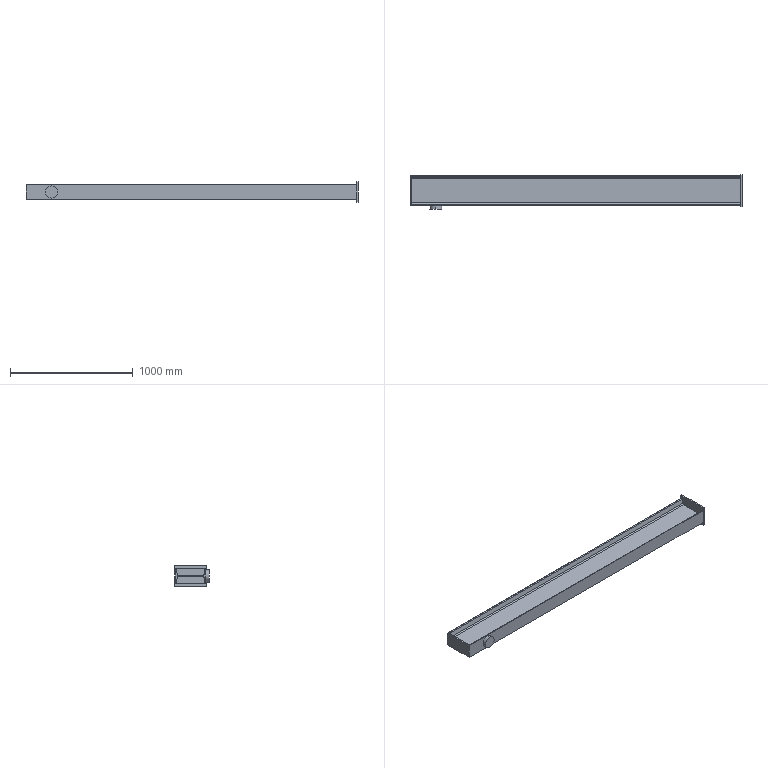Part | SolidWorks | features ICE 3, Fillet 2, Extrusion 1 | 1 solid | 30 faces | box 2710 x 284 x 170 mm | volume 14871084 mm3 | plane 20 | cylinder 10 | commonest cylinder face diameters 10 x4 20 x4 100 x2
STEP:
#1=CARTESIAN_POINT('',(205.,-28.,-50.));
#2=VERTEX_POINT('',#1);
#3=CARTESIAN_POINT('',(205.,-28.,50.));
#4=VERTEX_POINT('',#3);
#5=CARTESIAN_POINT('',(205.,-28.,0.));
#6=DIRECTION('',(0.,-1.,0.));
#7=DIRECTION('',(0.,0.,-1.));
#8=AXIS2_PLACEMENT_3D('',#5,#6,#7);
#9=CIRCLE('',#8,50.);
#10=EDGE_CURVE('',#2,#4,#9,.T.);
#11=ORIENTED_EDGE('',*,*,#10,.F.);
#12=CARTESIAN_POINT('',(205.,0.,-50.));
#13=VERTEX_POINT('',#12);
#14=CARTESIAN_POINT('',(205.,-28.,-50.));
#15=DIRECTION('',(0.,1.,0.));
#16=VECTOR('',#15,1000.);
#17=LINE('',#14,#16);
#18=EDGE_CURVE('',#2,#13,#17,.T.);
#19=ORIENTED_EDGE('',*,*,#18,.T.);
#20=CARTESIAN_POINT('',(205.,0.,50.));
#21=VERTEX_POINT('',#20);
#22=CARTESIAN_POINT('',(205.,0.,0.));
#23=DIRECTION('',(0.,-1.,0.));
#24=DIRECTION('',(0.,0.,1.));
#25=AXIS2_PLACEMENT_3D('',#22,#23,#24);
#26=CIRCLE('',#25,50.);
#27=EDGE_CURVE('',#13,#21,#26,.T.);
#28=ORIENTED_EDGE('',*,*,#27,.T.);
#29=CARTESIAN_POINT('',(205.,-28.,50.));
#30=DIRECTION('',(0.,1.,0.));
#31=VECTOR('',#30,1000.);
#32=LINE('',#29,#31);
#33=EDGE_CURVE('',#4,#21,#32,.T.);
#34=ORIENTED_EDGE('',*,*,#33,.F.);
#35=EDGE_LOOP('',(#11,#19,#28,#34));
#36=FACE_OUTER_BOUND('',#35,.T.);
#37=CARTESIAN_POINT('',(205.,-28.,0.));
#38=DIRECTION('',(0.,1.,0.));
#39=DIRECTION('',(0.,0.,1.));
#40=AXIS2_PLACEMENT_3D('',#37,#38,#39);
#41=CYLINDRICAL_SURFACE('',#40,50.);
#42=ADVANCED_FACE('',(#36),#41,.T.);
#43=CARTESIAN_POINT('',(2695.,8.363,-54.822));
#44=VERTEX_POINT('',#43);
#45=CARTESIAN_POINT('',(2695.,15.274,-13.356));
#46=VERTEX_POINT('',#45);
#47=CARTESIAN_POINT('',(2695.,16.667,-5.));
#48=DIRECTION('',(0.,0.1644,0.9864));
#49=VECTOR('',#48,1000.);
#50=LINE('',#47,#49);
#51=EDGE_CURVE('',#44,#46,#50,.T.);
#52=ORIENTED_EDGE('',*,*,#51,.F.);
#53=CARTESIAN_POINT('',(5.,8.363,-54.822));
#54=VERTEX_POINT('',#53);
#55=CARTESIAN_POINT('',(2700.,8.363,-54.822));
#56=DIRECTION('',(-1.,0.,0.));
#57=VECTOR('',#56,1000.);
#58=LINE('',#55,#57);
#59=EDGE_CURVE('',#44,#54,#58,.T.);
#60=ORIENTED_EDGE('',*,*,#59,.T.);
#61=CARTESIAN_POINT('',(5.,15.274,-13.356));
#62=VERTEX_POINT('',#61);
#63=CARTESIAN_POINT('',(5.,16.667,-5.));
#64=DIRECTION('',(0.,-0.1644,-0.9864));
#65=VECTOR('',#64,1000.);
#66=LINE('',#63,#65);
#67=EDGE_CURVE('',#62,#54,#66,.T.);
#68=ORIENTED_EDGE('',*,*,#67,.F.);
#69=CARTESIAN_POINT('',(2700.,15.274,-13.356));
#70=DIRECTION('',(1.,0.,0.));
#71=VECTOR('',#70,1000.);
#72=LINE('',#69,#71);
#73=EDGE_CURVE('',#62,#46,#72,.T.);
#74=ORIENTED_EDGE('',*,*,#73,.T.);
#75=EDGE_LOOP('',(#52,#60,#68,#74));
#76=FACE_OUTER_BOUND('',#75,.T.);
#77=CARTESIAN_POINT('',(2700.,16.667,-5.));
#78=DIRECTION('',(0.,-0.9864,0.1644));
#79=DIRECTION('',(0.,-0.1644,-0.9864));
#80=AXIS2_PLACEMENT_3D('',#77,#78,#79);
#81=PLANE('',#80);
#82=ADVANCED_FACE('',(#76),#81,.F.);
#83=CARTESIAN_POINT('',(2695.,25.138,-5.));
#84=VERTEX_POINT('',#83);
#85=CARTESIAN_POINT('',(2695.,224.862,-5.));
#86=VERTEX_POINT('',#85);
#87=CARTESIAN_POINT('',(2695.,233.333,-5.));
#88=DIRECTION('',(0.,1.,0.));
#89=VECTOR('',#88,1000.);
#90=LINE('',#87,#89);
#91=EDGE_CURVE('',#84,#86,#90,.T.);
#92=ORIENTED_EDGE('',*,*,#91,.F.);
#93=CARTESIAN_POINT('',(5.,25.138,-5.));
#94=VERTEX_POINT('',#93);
#95=CARTESIAN_POINT('',(0.,25.138,-5.));
#96=DIRECTION('',(-1.,0.,0.));
#97=VECTOR('',#96,1000.);
#98=LINE('',#95,#97);
#99=EDGE_CURVE('',#84,#94,#98,.T.);
#100=ORIENTED_EDGE('',*,*,#99,.T.);
#101=CARTESIAN_POINT('',(5.,224.862,-5.));
#102=VERTEX_POINT('',#101);
#103=CARTESIAN_POINT('',(5.,233.333,-5.));
#104=DIRECTION('',(0.,-1.,0.));
#105=VECTOR('',#104,1000.);
#106=LINE('',#103,#105);
#107=EDGE_CURVE('',#102,#94,#106,.T.);
#108=ORIENTED_EDGE('',*,*,#107,.F.);
#109=CARTESIAN_POINT('',(2700.,224.862,-5.));
#110=DIRECTION('',(1.,0.,0.));
#111=VECTOR('',#110,1000.);
#112=LINE('',#109,#111);
#113=EDGE_CURVE('',#102,#86,#112,.T.);
#114=ORIENTED_EDGE('',*,*,#113,.T.);
#115=EDGE_LOOP('',(#92,#100,#108,#114));
#116=FACE_OUTER_BOUND('',#115,.T.);
#117=CARTESIAN_POINT('',(2700.,233.333,-5.));
#118=DIRECTION('',(0.,0.,1.));
#119=DIRECTION('',(0.,-1.,0.));
#120=AXIS2_PLACEMENT_3D('',#117,#118,#119);
#121=PLANE('',#120);
#122=ADVANCED_FACE('',(#116),#121,.F.);
#123=CARTESIAN_POINT('',(2695.,234.726,-13.356));
#124=VERTEX_POINT('',#123);
#125=CARTESIAN_POINT('',(2695.,241.637,-54.822));
#126=VERTEX_POINT('',#125);
#127=CARTESIAN_POINT('',(2695.,242.333,-59.));
#128=DIRECTION('',(0.,0.1644,-0.9864));
#129=VECTOR('',#128,1000.);
#130=LINE('',#127,#129);
#131=EDGE_CURVE('',#124,#126,#130,.T.);
#132=ORIENTED_EDGE('',*,*,#131,.F.);
#133=CARTESIAN_POINT('',(5.,234.726,-13.356));
#134=VERTEX_POINT('',#133);
#135=CARTESIAN_POINT('',(0.,234.726,-13.356));
#136=DIRECTION('',(-1.,0.,0.));
#137=VECTOR('',#136,1000.);
#138=LINE('',#135,#137);
#139=EDGE_CURVE('',#124,#134,#138,.T.);
#140=ORIENTED_EDGE('',*,*,#139,.T.);
#141=CARTESIAN_POINT('',(5.,241.637,-54.822));
#142=VERTEX_POINT('',#141);
#143=CARTESIAN_POINT('',(5.,242.333,-59.));
#144=DIRECTION('',(0.,-0.1644,0.9864));
#145=VECTOR('',#144,1000.);
#146=LINE('',#143,#145);
#147=EDGE_CURVE('',#142,#134,#146,.T.);
#148=ORIENTED_EDGE('',*,*,#147,.F.);
#149=CARTESIAN_POINT('',(2700.,241.637,-54.822));
#150=DIRECTION('',(1.,0.,0.));
#151=VECTOR('',#150,1000.);
#152=LINE('',#149,#151);
#153=EDGE_CURVE('',#142,#126,#152,.T.);
#154=ORIENTED_EDGE('',*,*,#153,.T.);
#155=EDGE_LOOP('',(#132,#140,#148,#154));
#156=FACE_OUTER_BOUND('',#155,.T.);
#157=CARTESIAN_POINT('',(2700.,242.333,-59.));
#158=DIRECTION('',(0.,0.9864,0.1644));
#159=DIRECTION('',(0.,-0.1644,0.9864));
#160=AXIS2_PLACEMENT_3D('',#157,#158,#159);
#161=PLANE('',#160);
#162=ADVANCED_FACE('',(#156),#161,.F.);
#163=CARTESIAN_POINT('',(2695.,241.637,54.822));
#164=VERTEX_POINT('',#163);
#165=CARTESIAN_POINT('',(2695.,234.726,13.356));
#166=VERTEX_POINT('',#165);
#167=CARTESIAN_POINT('',(2695.,242.333,59.));
#168=DIRECTION('',(0.,-0.1644,-0.9864));
#169=VECTOR('',#168,1000.);
#170=LINE('',#167,#169);
#171=EDGE_CURVE('',#164,#166,#170,.T.);
#172=ORIENTED_EDGE('',*,*,#171,.F.);
#173=CARTESIAN_POINT('',(5.,241.637,54.822));
#174=VERTEX_POINT('',#173);
#175=CARTESIAN_POINT('',(2700.,241.637,54.822));
#176=DIRECTION('',(-1.,0.,0.));
#177=VECTOR('',#176,1000.);
#178=LINE('',#175,#177);
#179=EDGE_CURVE('',#164,#174,#178,.T.);
#180=ORIENTED_EDGE('',*,*,#179,.T.);
#181=CARTESIAN_POINT('',(5.,234.726,13.356));
#182=VERTEX_POINT('',#181);
#183=CARTESIAN_POINT('',(5.,242.333,59.));
#184=DIRECTION('',(0.,0.1644,0.9864));
#185=VECTOR('',#184,1000.);
#186=LINE('',#183,#185);
#187=EDGE_CURVE('',#182,#174,#186,.T.);
#188=ORIENTED_EDGE('',*,*,#187,.F.);
#189=CARTESIAN_POINT('',(2700.,234.726,13.356));
#190=DIRECTION('',(1.,0.,0.));
#191=VECTOR('',#190,1000.);
#192=LINE('',#189,#191);
#193=EDGE_CURVE('',#182,#166,#192,.T.);
#194=ORIENTED_EDGE('',*,*,#193,.T.);
#195=EDGE_LOOP('',(#172,#180,#188,#194));
#196=FACE_OUTER_BOUND('',#195,.T.);
#197=CARTESIAN_POINT('',(2700.,242.333,59.));
#198=DIRECTION('',(0.,0.9864,-0.1644));
#199=DIRECTION('',(0.,0.1644,0.9864));
#200=AXIS2_PLACEMENT_3D('',#197,#198,#199);
#201=PLANE('',#200);
#202=ADVANCED_FACE('',(#196),#201,.F.);
#203=CARTESIAN_POINT('',(2695.,224.862,5.));
#204=VERTEX_POINT('',#203);
#205=CARTESIAN_POINT('',(2695.,25.138,5.));
#206=VERTEX_POINT('',#205);
#207=CARTESIAN_POINT('',(2695.,233.333,5.));
#208=DIRECTION('',(0.,-1.,0.));
#209=VECTOR('',#208,1000.);
#210=LINE('',#207,#209);
#211=EDGE_CURVE('',#204,#206,#210,.T.);
#212=ORIENTED_EDGE('',*,*,#211,.F.);
#213=CARTESIAN_POINT('',(5.,224.862,5.));
#214=VERTEX_POINT('',#213);
#215=CARTESIAN_POINT('',(0.,224.862,5.));
#216=DIRECTION('',(-1.,0.,0.));
#217=VECTOR('',#216,1000.);
#218=LINE('',#215,#217);
#219=EDGE_CURVE('',#204,#214,#218,.T.);
#220=ORIENTED_EDGE('',*,*,#219,.T.);
#221=CARTESIAN_POINT('',(5.,25.138,5.));
#222=VERTEX_POINT('',#221);
#223=CARTESIAN_POINT('',(5.,233.333,5.));
#224=DIRECTION('',(0.,1.,0.));
#225=VECTOR('',#224,1000.);
#226=LINE('',#223,#225);
#227=EDGE_CURVE('',#222,#214,#226,.T.);
#228=ORIENTED_EDGE('',*,*,#227,.F.);
#229=CARTESIAN_POINT('',(2700.,25.138,5.));
#230=DIRECTION('',(1.,0.,0.));
#231=VECTOR('',#230,1000.);
#232=LINE('',#229,#231);
#233=EDGE_CURVE('',#222,#206,#232,.T.);
#234=ORIENTED_EDGE('',*,*,#233,.T.);
#235=EDGE_LOOP('',(#212,#220,#228,#234));
#236=FACE_OUTER_BOUND('',#235,.T.);
#237=CARTESIAN_POINT('',(2700.,233.333,5.));
#238=DIRECTION('',(0.,0.,-1.));
#239=DIRECTION('',(0.,1.,0.));
#240=AXIS2_PLACEMENT_3D('',#237,#238,#239);
#241=PLANE('',#240);
#242=ADVANCED_FACE('',(#236),#241,.F.);
#243=CARTESIAN_POINT('',(2695.,15.274,13.356));
#244=VERTEX_POINT('',#243);
#245=CARTESIAN_POINT('',(2695.,8.363,54.822));
#246=VERTEX_POINT('',#245);
#247=CARTESIAN_POINT('',(2695.,16.667,5.));
#248=DIRECTION('',(0.,-0.1644,0.9864));
#249=VECTOR('',#248,1000.);
#250=LINE('',#247,#249);
#251=EDGE_CURVE('',#244,#246,#250,.T.);
#252=ORIENTED_EDGE('',*,*,#251,.F.);
#253=CARTESIAN_POINT('',(5.,15.274,13.356));
#254=VERTEX_POINT('',#253);
#255=CARTESIAN_POINT('',(0.,15.274,13.356));
#256=DIRECTION('',(-1.,0.,0.));
#257=VECTOR('',#256,1000.);
#258=LINE('',#255,#257);
#259=EDGE_CURVE('',#244,#254,#258,.T.);
#260=ORIENTED_EDGE('',*,*,#259,.T.);
#261=CARTESIAN_POINT('',(5.,8.363,54.822));
#262=VERTEX_POINT('',#261);
#263=CARTESIAN_POINT('',(5.,16.667,5.));
#264=DIRECTION('',(0.,0.1644,-0.9864));
#265=VECTOR('',#264,1000.);
#266=LINE('',#263,#265);
#267=EDGE_CURVE('',#262,#254,#266,.T.);
#268=ORIENTED_EDGE('',*,*,#267,.F.);
#269=CARTESIAN_POINT('',(2700.,8.363,54.822));
#270=DIRECTION('',(1.,0.,0.));
#271=VECTOR('',#270,1000.);
#272=LINE('',#269,#271);
#273=EDGE_CURVE('',#262,#246,#272,.T.);
#274=ORIENTED_EDGE('',*,*,#273,.T.);
#275=EDGE_LOOP('',(#252,#260,#268,#274));
#276=FACE_OUTER_BOUND('',#275,.T.);
#277=CARTESIAN_POINT('',(2700.,16.667,5.));
#278=DIRECTION('',(0.,-0.9864,-0.1644));
#279=DIRECTION('',(0.,0.1644,-0.9864));
#280=AXIS2_PLACEMENT_3D('',#277,#278,#279);
#281=PLANE('',#280);
#282=ADVANCED_FACE('',(#276),#281,.F.);
#283=CARTESIAN_POINT('',(2695.,224.862,-15.));
#284=DIRECTION('',(-1.,0.,0.));
#285=DIRECTION('',(0.,0.,-1.));
#286=AXIS2_PLACEMENT_3D('',#283,#284,#285);
#287=CIRCLE('',#286,10.);
#288=EDGE_CURVE('',#86,#124,#287,.T.);
#289=ORIENTED_EDGE('',*,*,#288,.F.);
#290=ORIENTED_EDGE('',*,*,#113,.F.);
#291=CARTESIAN_POINT('',(5.,224.862,-15.));
#292=DIRECTION('',(1.,0.,0.));
#293=DIRECTION('',(0.,0.,1.));
#294=AXIS2_PLACEMENT_3D('',#291,#292,#293);
#295=CIRCLE('',#294,10.);
#296=EDGE_CURVE('',#134,#102,#295,.T.);
#297=ORIENTED_EDGE('',*,*,#296,.F.);
#298=ORIENTED_EDGE('',*,*,#139,.F.);
#299=EDGE_LOOP('',(#289,#290,#297,#298));
#300=FACE_OUTER_BOUND('',#299,.T.);
#301=CARTESIAN_POINT('',(2700.,224.862,-15.));
#302=DIRECTION('',(1.,0.,0.));
#303=DIRECTION('',(0.,0.,-1.));
#304=AXIS2_PLACEMENT_3D('',#301,#302,#303);
#305=CYLINDRICAL_SURFACE('',#304,10.);
#306=ADVANCED_FACE('',(#300),#305,.F.);
#307=CARTESIAN_POINT('',(2695.,25.138,-15.));
#308=DIRECTION('',(-1.,0.,0.));
#309=DIRECTION('',(0.,0.,-1.));
#310=AXIS2_PLACEMENT_3D('',#307,#308,#309);
#311=CIRCLE('',#310,10.);
#312=EDGE_CURVE('',#46,#84,#311,.T.);
#313=ORIENTED_EDGE('',*,*,#312,.F.);
#314=ORIENTED_EDGE('',*,*,#73,.F.);
#315=CARTESIAN_POINT('',(5.,25.138,-15.));
#316=DIRECTION('',(1.,0.,0.));
#317=DIRECTION('',(0.,0.,1.));
#318=AXIS2_PLACEMENT_3D('',#315,#316,#317);
#319=CIRCLE('',#318,10.);
#320=EDGE_CURVE('',#94,#62,#319,.T.);
#321=ORIENTED_EDGE('',*,*,#320,.F.);
#322=ORIENTED_EDGE('',*,*,#99,.F.);
#323=EDGE_LOOP('',(#313,#314,#321,#322));
#324=FACE_OUTER_BOUND('',#323,.T.);
#325=CARTESIAN_POINT('',(2700.,25.138,-15.));
#326=DIRECTION('',(1.,0.,0.));
#327=DIRECTION('',(0.,0.,-1.));
#328=AXIS2_PLACEMENT_3D('',#325,#326,#327);
#329=CYLINDRICAL_SURFACE('',#328,10.);
#330=ADVANCED_FACE('',(#324),#329,.F.);
#331=CARTESIAN_POINT('',(2695.,25.138,15.));
#332=DIRECTION('',(-1.,0.,0.));
#333=DIRECTION('',(0.,0.,-1.));
#334=AXIS2_PLACEMENT_3D('',#331,#332,#333);
#335=CIRCLE('',#334,10.);
#336=EDGE_CURVE('',#206,#244,#335,.T.);
#337=ORIENTED_EDGE('',*,*,#336,.F.);
#338=ORIENTED_EDGE('',*,*,#233,.F.);
#339=CARTESIAN_POINT('',(5.,25.138,15.));
#340=DIRECTION('',(1.,0.,0.));
#341=DIRECTION('',(0.,0.,1.));
#342=AXIS2_PLACEMENT_3D('',#339,#340,#341);
#343=CIRCLE('',#342,10.);
#344=EDGE_CURVE('',#254,#222,#343,.T.);
#345=ORIENTED_EDGE('',*,*,#344,.F.);
#346=ORIENTED_EDGE('',*,*,#259,.F.);
#347=EDGE_LOOP('',(#337,#338,#345,#346));
#348=FACE_OUTER_BOUND('',#347,.T.);
#349=CARTESIAN_POINT('',(2700.,25.138,15.));
#350=DIRECTION('',(1.,0.,0.));
#351=DIRECTION('',(0.,0.,-1.));
#352=AXIS2_PLACEMENT_3D('',#349,#350,#351);
#353=CYLINDRICAL_SURFACE('',#352,10.);
#354=ADVANCED_FACE('',(#348),#353,.F.);
#355=CARTESIAN_POINT('',(2695.,224.862,15.));
#356=DIRECTION('',(-1.,0.,0.));
#357=DIRECTION('',(0.,0.,-1.));
#358=AXIS2_PLACEMENT_3D('',#355,#356,#357);
#359=CIRCLE('',#358,10.);
#360=EDGE_CURVE('',#166,#204,#359,.T.);
#361=ORIENTED_EDGE('',*,*,#360,.F.);
#362=ORIENTED_EDGE('',*,*,#193,.F.);
#363=CARTESIAN_POINT('',(5.,224.862,15.));
#364=DIRECTION('',(1.,0.,0.));
#365=DIRECTION('',(0.,0.,1.));
#366=AXIS2_PLACEMENT_3D('',#363,#364,#365);
#367=CIRCLE('',#366,10.);
#368=EDGE_CURVE('',#214,#182,#367,.T.);
#369=ORIENTED_EDGE('',*,*,#368,.F.);
#370=ORIENTED_EDGE('',*,*,#219,.F.);
#371=EDGE_LOOP('',(#361,#362,#369,#370));
#372=FACE_OUTER_BOUND('',#371,.T.);
#373=CARTESIAN_POINT('',(2700.,224.862,15.));
#374=DIRECTION('',(1.,0.,0.));
#375=DIRECTION('',(0.,0.,-1.));
#376=AXIS2_PLACEMENT_3D('',#373,#374,#375);
#377=CYLINDRICAL_SURFACE('',#376,10.);
#378=ADVANCED_FACE('',(#372),#377,.F.);
#379=ORIENTED_EDGE('',*,*,#179,.F.);
#380=CARTESIAN_POINT('',(2695.,246.569,59.));
#381=VERTEX_POINT('',#380);
#382=CARTESIAN_POINT('',(2695.,246.569,54.));
#383=DIRECTION('',(-1.,0.,0.));
#384=DIRECTION('',(0.,0.,-1.));
#385=AXIS2_PLACEMENT_3D('',#382,#383,#384);
#386=CIRCLE('',#385,5.);
#387=EDGE_CURVE('',#164,#381,#386,.T.);
#388=ORIENTED_EDGE('',*,*,#387,.T.);
#389=CARTESIAN_POINT('',(5.,246.569,59.));
#390=VERTEX_POINT('',#389);
#391=CARTESIAN_POINT('',(2700.,246.569,59.));
#392=DIRECTION('',(1.,0.,0.));
#393=VECTOR('',#392,1000.);
#394=LINE('',#391,#393);
#395=EDGE_CURVE('',#390,#381,#394,.T.);
#396=ORIENTED_EDGE('',*,*,#395,.F.);
#397=CARTESIAN_POINT('',(5.,246.569,54.));
#398=DIRECTION('',(1.,0.,0.));
#399=DIRECTION('',(0.,0.,1.));
#400=AXIS2_PLACEMENT_3D('',#397,#398,#399);
#401=CIRCLE('',#400,5.);
#402=EDGE_CURVE('',#390,#174,#401,.T.);
#403=ORIENTED_EDGE('',*,*,#402,.T.);
#404=EDGE_LOOP('',(#379,#388,#396,#403));
#405=FACE_OUTER_BOUND('',#404,.T.);
#406=CARTESIAN_POINT('',(2700.,246.569,54.));
#407=DIRECTION('',(-1.,0.,0.));
#408=DIRECTION('',(0.,0.,1.));
#409=AXIS2_PLACEMENT_3D('',#406,#407,#408);
#410=CYLINDRICAL_SURFACE('',#409,5.);
#411=ADVANCED_FACE('',(#405),#410,.T.);
#412=CARTESIAN_POINT('',(2695.,3.431,59.));
#413=VERTEX_POINT('',#412);
#414=CARTESIAN_POINT('',(5.,3.431,59.));
#415=VERTEX_POINT('',#414);
#416=CARTESIAN_POINT('',(2700.,3.431,59.));
#417=DIRECTION('',(-1.,0.,0.));
#418=VECTOR('',#417,1000.);
#419=LINE('',#416,#418);
#420=EDGE_CURVE('',#413,#415,#419,.T.);
#421=ORIENTED_EDGE('',*,*,#420,.F.);
#422=CARTESIAN_POINT('',(2695.,3.431,54.));
#423=DIRECTION('',(-1.,0.,0.));
#424=DIRECTION('',(0.,0.,-1.));
#425=AXIS2_PLACEMENT_3D('',#422,#423,#424);
#426=CIRCLE('',#425,5.);
#427=EDGE_CURVE('',#413,#246,#426,.T.);
#428=ORIENTED_EDGE('',*,*,#427,.T.);
#429=ORIENTED_EDGE('',*,*,#273,.F.);
#430=CARTESIAN_POINT('',(5.,3.431,54.));
#431=DIRECTION('',(1.,0.,0.));
#432=DIRECTION('',(0.,0.,1.));
#433=AXIS2_PLACEMENT_3D('',#430,#431,#432);
#434=CIRCLE('',#433,5.);
#435=EDGE_CURVE('',#262,#415,#434,.T.);
#436=ORIENTED_EDGE('',*,*,#435,.T.);
#437=EDGE_LOOP('',(#421,#428,#429,#436));
#438=FACE_OUTER_BOUND('',#437,.T.);
#439=CARTESIAN_POINT('',(2700.,3.431,54.));
#440=DIRECTION('',(-1.,0.,0.));
#441=DIRECTION('',(0.,0.,1.));
#442=AXIS2_PLACEMENT_3D('',#439,#440,#441);
#443=CYLINDRICAL_SURFACE('',#442,5.);
#444=ADVANCED_FACE('',(#438),#443,.T.);
#445=ORIENTED_EDGE('',*,*,#59,.F.);
#446=CARTESIAN_POINT('',(2695.,3.431,-59.));
#447=VERTEX_POINT('',#446);
#448=CARTESIAN_POINT('',(2695.,3.431,-54.));
#449=DIRECTION('',(-1.,0.,0.));
#450=DIRECTION('',(0.,0.,-1.));
#451=AXIS2_PLACEMENT_3D('',#448,#449,#450);
#452=CIRCLE('',#451,5.);
#453=EDGE_CURVE('',#44,#447,#452,.T.);
#454=ORIENTED_EDGE('',*,*,#453,.T.);
#455=CARTESIAN_POINT('',(5.,3.431,-59.));
#456=VERTEX_POINT('',#455);
#457=CARTESIAN_POINT('',(2700.,3.431,-59.));
#458=DIRECTION('',(1.,0.,0.));
#459=VECTOR('',#458,1000.);
#460=LINE('',#457,#459);
#461=EDGE_CURVE('',#456,#447,#460,.T.);
#462=ORIENTED_EDGE('',*,*,#461,.F.);
#463=CARTESIAN_POINT('',(5.,3.431,-54.));
#464=DIRECTION('',(1.,0.,0.));
#465=DIRECTION('',(0.,0.,1.));
#466=AXIS2_PLACEMENT_3D('',#463,#464,#465);
#467=CIRCLE('',#466,5.);
#468=EDGE_CURVE('',#456,#54,#467,.T.);
#469=ORIENTED_EDGE('',*,*,#468,.T.);
#470=EDGE_LOOP('',(#445,#454,#462,#469));
#471=FACE_OUTER_BOUND('',#470,.T.);
#472=CARTESIAN_POINT('',(2700.,3.431,-54.));
#473=DIRECTION('',(-1.,0.,0.));
#474=DIRECTION('',(0.,0.,1.));
#475=AXIS2_PLACEMENT_3D('',#472,#473,#474);
#476=CYLINDRICAL_SURFACE('',#475,5.);
#477=ADVANCED_FACE('',(#471),#476,.T.);
#478=CARTESIAN_POINT('',(2695.,246.569,-59.));
#479=VERTEX_POINT('',#478);
#480=CARTESIAN_POINT('',(5.,246.569,-59.));
#481=VERTEX_POINT('',#480);
#482=CARTESIAN_POINT('',(2700.,246.569,-59.));
#483=DIRECTION('',(-1.,0.,0.));
#484=VECTOR('',#483,1000.);
#485=LINE('',#482,#484);
#486=EDGE_CURVE('',#479,#481,#485,.T.);
#487=ORIENTED_EDGE('',*,*,#486,.F.);
#488=CARTESIAN_POINT('',(2695.,246.569,-54.));
#489=DIRECTION('',(-1.,0.,0.));
#490=DIRECTION('',(0.,0.,-1.));
#491=AXIS2_PLACEMENT_3D('',#488,#489,#490);
#492=CIRCLE('',#491,5.);
#493=EDGE_CURVE('',#479,#126,#492,.T.);
#494=ORIENTED_EDGE('',*,*,#493,.T.);
#495=ORIENTED_EDGE('',*,*,#153,.F.);
#496=CARTESIAN_POINT('',(5.,246.569,-54.));
#497=DIRECTION('',(1.,0.,0.));
#498=DIRECTION('',(0.,0.,1.));
#499=AXIS2_PLACEMENT_3D('',#496,#497,#498);
#500=CIRCLE('',#499,5.);
#501=EDGE_CURVE('',#142,#481,#500,.T.);
#502=ORIENTED_EDGE('',*,*,#501,.T.);
#503=EDGE_LOOP('',(#487,#494,#495,#502));
#504=FACE_OUTER_BOUND('',#503,.T.);
#505=CARTESIAN_POINT('',(2700.,246.569,-54.));
#506=DIRECTION('',(-1.,0.,0.));
#507=DIRECTION('',(0.,0.,1.));
#508=AXIS2_PLACEMENT_3D('',#505,#506,#507);
#509=CYLINDRICAL_SURFACE('',#508,5.);
#510=ADVANCED_FACE('',(#504),#509,.T.);
#511=CARTESIAN_POINT('',(205.,0.,0.));
#512=DIRECTION('',(0.,-1.,0.));
#513=DIRECTION('',(0.,0.,1.));
#514=AXIS2_PLACEMENT_3D('',#511,#512,#513);
#515=CIRCLE('',#514,50.);
#516=EDGE_CURVE('',#21,#13,#515,.T.);
#517=ORIENTED_EDGE('',*,*,#516,.F.);
#518=ORIENTED_EDGE('',*,*,#27,.F.);
#519=EDGE_LOOP('',(#517,#518));
#520=FACE_BOUND('',#519,.T.);
#521=CARTESIAN_POINT('',(2695.,0.,59.));
#522=VERTEX_POINT('',#521);
#523=CARTESIAN_POINT('',(2695.,0.,-59.));
#524=VERTEX_POINT('',#523);
#525=CARTESIAN_POINT('',(2695.,0.,59.));
#526=DIRECTION('',(0.,0.,-1.));
#527=VECTOR('',#526,1000.);
#528=LINE('',#525,#527);
#529=EDGE_CURVE('',#522,#524,#528,.T.);
#530=ORIENTED_EDGE('',*,*,#529,.F.);
#531=CARTESIAN_POINT('',(-5.,0.,59.));
#532=VERTEX_POINT('',#531);
#533=CARTESIAN_POINT('',(2700.,0.,59.));
#534=DIRECTION('',(-1.,0.,0.));
#535=VECTOR('',#534,1000.);
#536=LINE('',#533,#535);
#537=EDGE_CURVE('',#522,#532,#536,.T.);
#538=ORIENTED_EDGE('',*,*,#537,.T.);
#539=CARTESIAN_POINT('',(-5.,0.,-59.));
#540=VERTEX_POINT('',#539);
#541=CARTESIAN_POINT('',(-5.,0.,-59.));
#542=DIRECTION('',(0.,0.,1.));
#543=VECTOR('',#542,1000.);
#544=LINE('',#541,#543);
#545=EDGE_CURVE('',#540,#532,#544,.T.);
#546=ORIENTED_EDGE('',*,*,#545,.F.);
#547=CARTESIAN_POINT('',(2700.,0.,-59.));
#548=DIRECTION('',(-1.,0.,0.));
#549=VECTOR('',#548,1000.);
#550=LINE('',#547,#549);
#551=EDGE_CURVE('',#524,#540,#550,.T.);
#552=ORIENTED_EDGE('',*,*,#551,.F.);
#553=EDGE_LOOP('',(#530,#538,#546,#552));
#554=FACE_OUTER_BOUND('',#553,.T.);
#555=CARTESIAN_POINT('',(2700.,0.,59.));
#556=DIRECTION('',(0.,1.,0.));
#557=DIRECTION('',(0.,0.,1.));
#558=AXIS2_PLACEMENT_3D('',#555,#556,#557);
#559=PLANE('',#558);
#560=ADVANCED_FACE('',(#520,#554),#559,.F.);
#561=CARTESIAN_POINT('',(2695.,250.,-59.));
#562=DIRECTION('',(0.,1.,0.));
#563=VECTOR('',#562,1000.);
#564=LINE('',#561,#563);
#565=EDGE_CURVE('',#524,#447,#564,.T.);
#566=ORIENTED_EDGE('',*,*,#565,.F.);
#567=ORIENTED_EDGE('',*,*,#551,.T.);
#568=CARTESIAN_POINT('',(-5.,250.,-59.));
#569=VERTEX_POINT('',#568);
#570=CARTESIAN_POINT('',(-5.,250.,-59.));
#571=DIRECTION('',(0.,-1.,0.));
#572=VECTOR('',#571,1000.);
#573=LINE('',#570,#572);
#574=EDGE_CURVE('',#569,#540,#573,.T.);
#575=ORIENTED_EDGE('',*,*,#574,.F.);
#576=CARTESIAN_POINT('',(2695.,250.,-59.));
#577=VERTEX_POINT('',#576);
#578=CARTESIAN_POINT('',(2700.,250.,-59.));
#579=DIRECTION('',(-1.,0.,0.));
#580=VECTOR('',#579,1000.);
#581=LINE('',#578,#580);
#582=EDGE_CURVE('',#577,#569,#581,.T.);
#583=ORIENTED_EDGE('',*,*,#582,.F.);
#584=CARTESIAN_POINT('',(2695.,250.,-59.));
#585=DIRECTION('',(0.,1.,0.));
#586=VECTOR('',#585,1000.);
#587=LINE('',#584,#586);
#588=EDGE_CURVE('',#479,#577,#587,.T.);
#589=ORIENTED_EDGE('',*,*,#588,.F.);
#590=ORIENTED_EDGE('',*,*,#486,.T.);
#591=CARTESIAN_POINT('',(5.,250.,-59.));
#592=DIRECTION('',(0.,-1.,0.));
#593=VECTOR('',#592,1000.);
#594=LINE('',#591,#593);
#595=EDGE_CURVE('',#481,#456,#594,.T.);
#596=ORIENTED_EDGE('',*,*,#595,.T.);
#597=ORIENTED_EDGE('',*,*,#461,.T.);
#598=EDGE_LOOP('',(#566,#567,#575,#583,#589,#590,#596,#597));
#599=FACE_OUTER_BOUND('',#598,.T.);
#600=CARTESIAN_POINT('',(2700.,250.,-59.));
#601=DIRECTION('',(0.,0.,1.));
#602=DIRECTION('',(0.,-1.,0.));
#603=AXIS2_PLACEMENT_3D('',#600,#601,#602);
#604=PLANE('',#603);
#605=ADVANCED_FACE('',(#599),#604,.F.);
#606=CARTESIAN_POINT('',(2695.,250.,59.));
#607=VERTEX_POINT('',#606);
#608=CARTESIAN_POINT('',(2695.,250.,59.));
#609=DIRECTION('',(0.,0.,1.));
#610=VECTOR('',#609,1000.);
#611=LINE('',#608,#610);
#612=EDGE_CURVE('',#577,#607,#611,.T.);
#613=ORIENTED_EDGE('',*,*,#612,.F.);
#614=ORIENTED_EDGE('',*,*,#582,.T.);
#615=CARTESIAN_POINT('',(-5.,250.,59.));
#616=VERTEX_POINT('',#615);
#617=CARTESIAN_POINT('',(-5.,250.,-59.));
#618=DIRECTION('',(0.,0.,-1.));
#619=VECTOR('',#618,1000.);
#620=LINE('',#617,#619);
#621=EDGE_CURVE('',#616,#569,#620,.T.);
#622=ORIENTED_EDGE('',*,*,#621,.F.);
#623=CARTESIAN_POINT('',(2700.,250.,59.));
#624=DIRECTION('',(-1.,0.,0.));
#625=VECTOR('',#624,1000.);
#626=LINE('',#623,#625);
#627=EDGE_CURVE('',#607,#616,#626,.T.);
#628=ORIENTED_EDGE('',*,*,#627,.F.);
#629=EDGE_LOOP('',(#613,#614,#622,#628));
#630=FACE_OUTER_BOUND('',#629,.T.);
#631=CARTESIAN_POINT('',(2700.,250.,59.));
#632=DIRECTION('',(0.,-1.,0.));
#633=DIRECTION('',(0.,0.,-1.));
#634=AXIS2_PLACEMENT_3D('',#631,#632,#633);
#635=PLANE('',#634);
#636=ADVANCED_FACE('',(#630),#635,.F.);
#637=CARTESIAN_POINT('',(2695.,250.,59.));
#638=DIRECTION('',(0.,-1.,0.));
#639=VECTOR('',#638,1000.);
#640=LINE('',#637,#639);
#641=EDGE_CURVE('',#607,#381,#640,.T.);
#642=ORIENTED_EDGE('',*,*,#641,.F.);
#643=ORIENTED_EDGE('',*,*,#627,.T.);
#644=CARTESIAN_POINT('',(-5.,250.,59.));
#645=DIRECTION('',(0.,1.,0.));
#646=VECTOR('',#645,1000.);
#647=LINE('',#644,#646);
#648=EDGE_CURVE('',#532,#616,#647,.T.);
#649=ORIENTED_EDGE('',*,*,#648,.F.);
#650=ORIENTED_EDGE('',*,*,#537,.F.);
#651=CARTESIAN_POINT('',(2695.,250.,59.));
#652=DIRECTION('',(0.,-1.,0.));
#653=VECTOR('',#652,1000.);
#654=LINE('',#651,#653);
#655=EDGE_CURVE('',#413,#522,#654,.T.);
#656=ORIENTED_EDGE('',*,*,#655,.F.);
#657=ORIENTED_EDGE('',*,*,#420,.T.);
#658=CARTESIAN_POINT('',(5.,250.,59.));
#659=DIRECTION('',(0.,1.,0.));
#660=VECTOR('',#659,1000.);
#661=LINE('',#658,#660);
#662=EDGE_CURVE('',#415,#390,#661,.T.);
#663=ORIENTED_EDGE('',*,*,#662,.T.);
#664=ORIENTED_EDGE('',*,*,#395,.T.);
#665=EDGE_LOOP('',(#642,#643,#649,#650,#656,#657,#663,#664));
#666=FACE_OUTER_BOUND('',#665,.T.);
#667=CARTESIAN_POINT('',(2700.,250.,59.));
#668=DIRECTION('',(0.,0.,-1.));
#669=DIRECTION('',(-1.,0.,0.));
#670=AXIS2_PLACEMENT_3D('',#667,#668,#669);
#671=PLANE('',#670);
#672=ADVANCED_FACE('',(#666),#671,.F.);
#673=ORIENTED_EDGE('',*,*,#402,.F.);
#674=ORIENTED_EDGE('',*,*,#662,.F.);
#675=ORIENTED_EDGE('',*,*,#435,.F.);
#676=ORIENTED_EDGE('',*,*,#267,.T.);
#677=ORIENTED_EDGE('',*,*,#344,.T.);
#678=ORIENTED_EDGE('',*,*,#227,.T.);
#679=ORIENTED_EDGE('',*,*,#368,.T.);
#680=ORIENTED_EDGE('',*,*,#187,.T.);
#681=EDGE_LOOP('',(#673,#674,#675,#676,#677,#678,#679,#680));
#682=FACE_OUTER_BOUND('',#681,.T.);
#683=CARTESIAN_POINT('',(5.,0.,0.));
#684=DIRECTION('',(-1.,0.,0.));
#685=DIRECTION('',(0.,0.,1.));
#686=AXIS2_PLACEMENT_3D('',#683,#684,#685);
#687=PLANE('',#686);
#688=ADVANCED_FACE('',(#682),#687,.F.);
#689=ORIENTED_EDGE('',*,*,#574,.T.);
#690=ORIENTED_EDGE('',*,*,#545,.T.);
#691=ORIENTED_EDGE('',*,*,#648,.T.);
#692=ORIENTED_EDGE('',*,*,#621,.T.);
#693=EDGE_LOOP('',(#689,#690,#691,#692));
#694=FACE_OUTER_BOUND('',#693,.T.);
#695=CARTESIAN_POINT('',(-5.,0.,0.));
#696=DIRECTION('',(-1.,0.,0.));
#697=DIRECTION('',(0.,0.,1.));
#698=AXIS2_PLACEMENT_3D('',#695,#696,#697);
#699=PLANE('',#698);
#700=ADVANCED_FACE('',(#694),#699,.T.);
#701=ORIENTED_EDGE('',*,*,#468,.F.);
#702=ORIENTED_EDGE('',*,*,#595,.F.);
#703=ORIENTED_EDGE('',*,*,#501,.F.);
#704=ORIENTED_EDGE('',*,*,#147,.T.);
#705=ORIENTED_EDGE('',*,*,#296,.T.);
#706=ORIENTED_EDGE('',*,*,#107,.T.);
#707=ORIENTED_EDGE('',*,*,#320,.T.);
#708=ORIENTED_EDGE('',*,*,#67,.T.);
#709=EDGE_LOOP('',(#701,#702,#703,#704,#705,#706,#707,#708));
#710=FACE_OUTER_BOUND('',#709,.T.);
#711=CARTESIAN_POINT('',(5.,0.,0.));
#712=DIRECTION('',(-1.,0.,0.));
#713=DIRECTION('',(0.,0.,1.));
#714=AXIS2_PLACEMENT_3D('',#711,#712,#713);
#715=PLANE('',#714);
#716=ADVANCED_FACE('',(#710),#715,.F.);
#717=CARTESIAN_POINT('',(2695.,256.,85.));
#718=VERTEX_POINT('',#717);
#719=CARTESIAN_POINT('',(2695.,-6.,85.));
#720=VERTEX_POINT('',#719);
#721=CARTESIAN_POINT('',(2695.,256.,85.));
#722=DIRECTION('',(0.,-1.,0.));
#723=VECTOR('',#722,1000.);
#724=LINE('',#721,#723);
#725=EDGE_CURVE('',#718,#720,#724,.T.);
#726=ORIENTED_EDGE('',*,*,#725,.T.);
#727=CARTESIAN_POINT('',(2705.,-6.,85.));
#728=VERTEX_POINT('',#727);
#729=CARTESIAN_POINT('',(2705.,-6.,85.));
#730=DIRECTION('',(-1.,0.,0.));
#731=VECTOR('',#730,1000.);
#732=LINE('',#729,#731);
#733=EDGE_CURVE('',#728,#720,#732,.T.);
#734=ORIENTED_EDGE('',*,*,#733,.F.);
#735=CARTESIAN_POINT('',(2705.,256.,85.));
#736=VERTEX_POINT('',#735);
#737=CARTESIAN_POINT('',(2705.,256.,85.));
#738=DIRECTION('',(0.,-1.,0.));
#739=VECTOR('',#738,1000.);
#740=LINE('',#737,#739);
#741=EDGE_CURVE('',#736,#728,#740,.T.);
#742=ORIENTED_EDGE('',*,*,#741,.F.);
#743=CARTESIAN_POINT('',(2705.,256.,85.));
#744=DIRECTION('',(-1.,0.,0.));
#745=VECTOR('',#744,1000.);
#746=LINE('',#743,#745);
#747=EDGE_CURVE('',#736,#718,#746,.T.);
#748=ORIENTED_EDGE('',*,*,#747,.T.);
#749=EDGE_LOOP('',(#726,#734,#742,#748));
#750=FACE_OUTER_BOUND('',#749,.T.);
#751=CARTESIAN_POINT('',(2705.,256.,85.));
#752=DIRECTION('',(0.,0.,-1.));
#753=DIRECTION('',(0.,1.,0.));
#754=AXIS2_PLACEMENT_3D('',#751,#752,#753);
#755=PLANE('',#754);
#756=ADVANCED_FACE('',(#750),#755,.F.);
#757=CARTESIAN_POINT('',(2695.,-6.,-85.));
#758=VERTEX_POINT('',#757);
#759=CARTESIAN_POINT('',(2695.,-6.,85.));
#760=DIRECTION('',(0.,0.,-1.));
#761=VECTOR('',#760,1000.);
#762=LINE('',#759,#761);
#763=EDGE_CURVE('',#720,#758,#762,.T.);
#764=ORIENTED_EDGE('',*,*,#763,.T.);
#765=CARTESIAN_POINT('',(2705.,-6.,-85.));
#766=VERTEX_POINT('',#765);
#767=CARTESIAN_POINT('',(2705.,-6.,-85.));
#768=DIRECTION('',(-1.,0.,0.));
#769=VECTOR('',#768,1000.);
#770=LINE('',#767,#769);
#771=EDGE_CURVE('',#766,#758,#770,.T.);
#772=ORIENTED_EDGE('',*,*,#771,.F.);
#773=CARTESIAN_POINT('',(2705.,-6.,85.));
#774=DIRECTION('',(0.,0.,-1.));
#775=VECTOR('',#774,1000.);
#776=LINE('',#773,#775);
#777=EDGE_CURVE('',#728,#766,#776,.T.);
#778=ORIENTED_EDGE('',*,*,#777,.F.);
#779=ORIENTED_EDGE('',*,*,#733,.T.);
#780=EDGE_LOOP('',(#764,#772,#778,#779));
#781=FACE_OUTER_BOUND('',#780,.T.);
#782=CARTESIAN_POINT('',(2705.,-6.,85.));
#783=DIRECTION('',(0.,1.,0.));
#784=DIRECTION('',(0.,0.,1.));
#785=AXIS2_PLACEMENT_3D('',#782,#783,#784);
#786=PLANE('',#785);
#787=ADVANCED_FACE('',(#781),#786,.F.);
#788=CARTESIAN_POINT('',(2695.,256.,-85.));
#789=VERTEX_POINT('',#788);
#790=CARTESIAN_POINT('',(2695.,256.,-85.));
#791=DIRECTION('',(0.,1.,0.));
#792=VECTOR('',#791,1000.);
#793=LINE('',#790,#792);
#794=EDGE_CURVE('',#758,#789,#793,.T.);
#795=ORIENTED_EDGE('',*,*,#794,.T.);
#796=CARTESIAN_POINT('',(2705.,256.,-85.));
#797=VERTEX_POINT('',#796);
#798=CARTESIAN_POINT('',(2705.,256.,-85.));
#799=DIRECTION('',(-1.,0.,0.));
#800=VECTOR('',#799,1000.);
#801=LINE('',#798,#800);
#802=EDGE_CURVE('',#797,#789,#801,.T.);
#803=ORIENTED_EDGE('',*,*,#802,.F.);
#804=CARTESIAN_POINT('',(2705.,256.,-85.));
#805=DIRECTION('',(0.,1.,0.));
#806=VECTOR('',#805,1000.);
#807=LINE('',#804,#806);
#808=EDGE_CURVE('',#766,#797,#807,.T.);
#809=ORIENTED_EDGE('',*,*,#808,.F.);
#810=ORIENTED_EDGE('',*,*,#771,.T.);
#811=EDGE_LOOP('',(#795,#803,#809,#810));
#812=FACE_OUTER_BOUND('',#811,.T.);
#813=CARTESIAN_POINT('',(2705.,256.,-85.));
#814=DIRECTION('',(0.,0.,1.));
#815=DIRECTION('',(0.,-1.,0.));
#816=AXIS2_PLACEMENT_3D('',#813,#814,#815);
#817=PLANE('',#816);
#818=ADVANCED_FACE('',(#812),#817,.F.);
#819=CARTESIAN_POINT('',(2695.,256.,85.));
#820=DIRECTION('',(0.,0.,1.));
#821=VECTOR('',#820,1000.);
#822=LINE('',#819,#821);
#823=EDGE_CURVE('',#789,#718,#822,.T.);
#824=ORIENTED_EDGE('',*,*,#823,.T.);
#825=ORIENTED_EDGE('',*,*,#747,.F.);
#826=CARTESIAN_POINT('',(2705.,256.,85.));
#827=DIRECTION('',(0.,0.,1.));
#828=VECTOR('',#827,1000.);
#829=LINE('',#826,#828);
#830=EDGE_CURVE('',#797,#736,#829,.T.);
#831=ORIENTED_EDGE('',*,*,#830,.F.);
#832=ORIENTED_EDGE('',*,*,#802,.T.);
#833=EDGE_LOOP('',(#824,#825,#831,#832));
#834=FACE_OUTER_BOUND('',#833,.T.);
#835=CARTESIAN_POINT('',(2705.,256.,85.));
#836=DIRECTION('',(0.,-1.,0.));
#837=DIRECTION('',(0.,0.,-1.));
#838=AXIS2_PLACEMENT_3D('',#835,#836,#837);
#839=PLANE('',#838);
#840=ADVANCED_FACE('',(#834),#839,.F.);
#841=ORIENTED_EDGE('',*,*,#741,.T.);
#842=ORIENTED_EDGE('',*,*,#777,.T.);
#843=ORIENTED_EDGE('',*,*,#808,.T.);
#844=ORIENTED_EDGE('',*,*,#830,.T.);
#845=EDGE_LOOP('',(#841,#842,#843,#844));
#846=FACE_OUTER_BOUND('',#845,.T.);
#847=CARTESIAN_POINT('',(2705.,0.,0.));
#848=DIRECTION('',(1.,0.,0.));
#849=DIRECTION('',(0.,0.,-1.));
#850=AXIS2_PLACEMENT_3D('',#847,#848,#849);
#851=PLANE('',#850);
#852=ADVANCED_FACE('',(#846),#851,.T.);
#853=ORIENTED_EDGE('',*,*,#493,.F.);
#854=ORIENTED_EDGE('',*,*,#588,.T.);
#855=ORIENTED_EDGE('',*,*,#612,.T.);
#856=ORIENTED_EDGE('',*,*,#641,.T.);
#857=ORIENTED_EDGE('',*,*,#387,.F.);
#858=ORIENTED_EDGE('',*,*,#171,.T.);
#859=ORIENTED_EDGE('',*,*,#360,.T.);
#860=ORIENTED_EDGE('',*,*,#211,.T.);
#861=ORIENTED_EDGE('',*,*,#336,.T.);
#862=ORIENTED_EDGE('',*,*,#251,.T.);
#863=ORIENTED_EDGE('',*,*,#427,.F.);
#864=ORIENTED_EDGE('',*,*,#655,.T.);
#865=ORIENTED_EDGE('',*,*,#529,.T.);
#866=ORIENTED_EDGE('',*,*,#565,.T.);
#867=ORIENTED_EDGE('',*,*,#453,.F.);
#868=ORIENTED_EDGE('',*,*,#51,.T.);
#869=ORIENTED_EDGE('',*,*,#312,.T.);
#870=ORIENTED_EDGE('',*,*,#91,.T.);
#871=ORIENTED_EDGE('',*,*,#288,.T.);
#872=ORIENTED_EDGE('',*,*,#131,.T.);
#873=EDGE_LOOP('',(#853,#854,#855,#856,#857,#858,#859,#860,#861,#862,#863,#864,#865,#866,#867,#868,#869,#870,#871,#872));
#874=FACE_BOUND('',#873,.T.);
#875=ORIENTED_EDGE('',*,*,#725,.F.);
#876=ORIENTED_EDGE('',*,*,#823,.F.);
#877=ORIENTED_EDGE('',*,*,#794,.F.);
#878=ORIENTED_EDGE('',*,*,#763,.F.);
#879=EDGE_LOOP('',(#875,#876,#877,#878));
#880=FACE_OUTER_BOUND('',#879,.T.);
#881=CARTESIAN_POINT('',(2695.,0.,0.));
#882=DIRECTION('',(1.,0.,0.));
#883=DIRECTION('',(0.,0.,-1.));
#884=AXIS2_PLACEMENT_3D('',#881,#882,#883);
#885=PLANE('',#884);
#886=ADVANCED_FACE('',(#874,#880),#885,.F.);
#887=ORIENTED_EDGE('',*,*,#18,.F.);
#888=CARTESIAN_POINT('',(205.,-28.,0.));
#889=DIRECTION('',(0.,-1.,0.));
#890=DIRECTION('',(0.,0.,-1.));
#891=AXIS2_PLACEMENT_3D('',#888,#889,#890);
#892=CIRCLE('',#891,50.);
#893=EDGE_CURVE('',#4,#2,#892,.T.);
#894=ORIENTED_EDGE('',*,*,#893,.F.);
#895=ORIENTED_EDGE('',*,*,#33,.T.);
#896=ORIENTED_EDGE('',*,*,#516,.T.);
#897=EDGE_LOOP('',(#887,#894,#895,#896));
#898=FACE_OUTER_BOUND('',#897,.T.);
#899=CARTESIAN_POINT('',(205.,-28.,0.));
#900=DIRECTION('',(0.,1.,0.));
#901=DIRECTION('',(0.,0.,1.));
#902=AXIS2_PLACEMENT_3D('',#899,#900,#901);
#903=CYLINDRICAL_SURFACE('',#902,50.);
#904=ADVANCED_FACE('',(#898),#903,.T.);
#905=ORIENTED_EDGE('',*,*,#893,.T.);
#906=ORIENTED_EDGE('',*,*,#10,.T.);
#907=EDGE_LOOP('',(#905,#906));
#908=FACE_OUTER_BOUND('',#907,.T.);
#909=CARTESIAN_POINT('',(205.,-28.,0.));
#910=DIRECTION('',(0.,-1.,0.));
#911=DIRECTION('',(0.,0.,-1.));
#912=AXIS2_PLACEMENT_3D('',#909,#910,#911);
#913=PLANE('',#912);
#914=ADVANCED_FACE('',(#908),#913,.T.);
#915=CLOSED_SHELL('',(#42,#82,#122,#162,#202,#242,#282,#306,#330,#354,#378,#411,#444,#477,#510,#560,#605,#636,#672,#688,#700,#716,#756,#787,#818,#840,#852,#886,#904,#914));
#916=MANIFOLD_SOLID_BREP('',#915);
#917=CARTESIAN_POINT('',(0.,0.,0.));
#918=DIRECTION('',(0.,0.,1.));
#919=DIRECTION('',(1.,0.,0.));
#920=AXIS2_PLACEMENT_3D('',#917,#918,#919);
#921=(LENGTH_UNIT()NAMED_UNIT(*)SI_UNIT(.MILLI.,.METRE.));
#922=UNCERTAINTY_MEASURE_WITH_UNIT(LENGTH_MEASURE(0.00001),#921,'','');
#923=(NAMED_UNIT(*)PLANE_ANGLE_UNIT()SI_UNIT($,.RADIAN.));
#924=(NAMED_UNIT(*)SI_UNIT($,.STERADIAN.)SOLID_ANGLE_UNIT());
#925=(GEOMETRIC_REPRESENTATION_CONTEXT(3)GLOBAL_UNCERTAINTY_ASSIGNED_CONTEXT((#922))GLOBAL_UNIT_ASSIGNED_CONTEXT((#921,#923,#924))REPRESENTATION_CONTEXT('',''));
#926=ADVANCED_BREP_SHAPE_REPRESENTATION('',(#916,#920),#925);